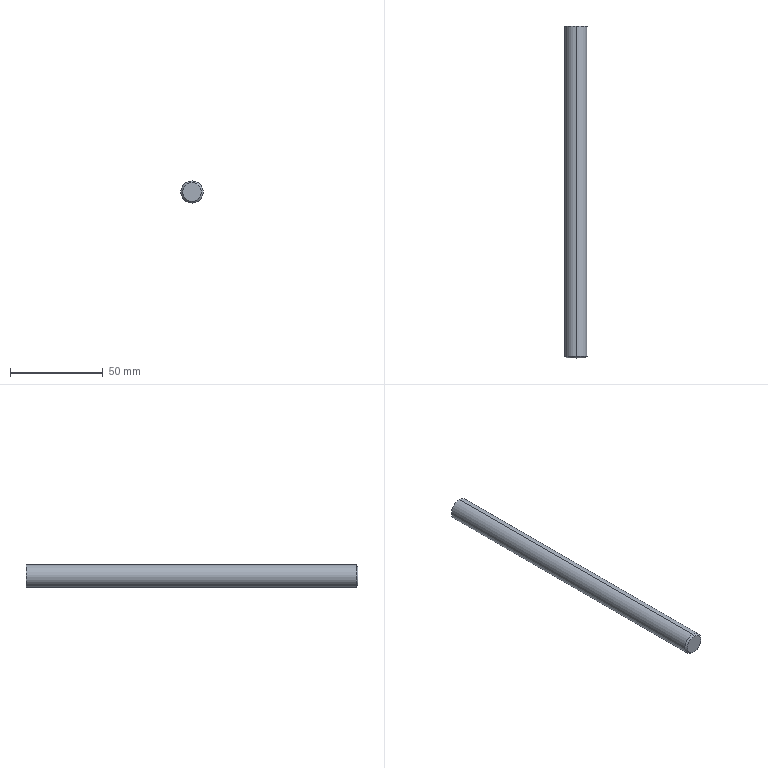Part | SolidWorks | features Chamfer 1, Extrusion 1, HoleWzd 1 | 1 solid | 10 faces | box 12 x 179 x 12 mm | volume 19967 mm3 | cone 4 | cylinder 4 | plane 2 | commonest cylinder face diameters 3.3 x2 12 x2
STEP:
#1=CARTESIAN_POINT('',(0.,0.,-5.));
#2=VERTEX_POINT('',#1);
#3=CARTESIAN_POINT('',(0.,0.,5.));
#4=VERTEX_POINT('',#3);
#5=CARTESIAN_POINT('',(0.,0.,0.));
#6=DIRECTION('',(0.,-1.,0.));
#7=DIRECTION('',(0.,0.,1.));
#8=AXIS2_PLACEMENT_3D('',#5,#6,#7);
#9=CIRCLE('',#8,5.);
#10=EDGE_CURVE('',#2,#4,#9,.T.);
#11=ORIENTED_EDGE('',*,*,#10,.F.);
#12=CARTESIAN_POINT('',(0.,1.,-6.));
#13=VERTEX_POINT('',#12);
#14=CARTESIAN_POINT('',(0.,1.,-6.));
#15=DIRECTION('',(0.,0.7071,-0.7071));
#16=VECTOR('',#15,1000.);
#17=LINE('',#14,#16);
#18=EDGE_CURVE('',#2,#13,#17,.T.);
#19=ORIENTED_EDGE('',*,*,#18,.T.);
#20=CARTESIAN_POINT('',(0.,1.,6.));
#21=VERTEX_POINT('',#20);
#22=CARTESIAN_POINT('',(0.,1.,0.));
#23=DIRECTION('',(0.,1.,0.));
#24=DIRECTION('',(0.,0.,1.));
#25=AXIS2_PLACEMENT_3D('',#22,#23,#24);
#26=CIRCLE('',#25,6.);
#27=EDGE_CURVE('',#21,#13,#26,.T.);
#28=ORIENTED_EDGE('',*,*,#27,.F.);
#29=CARTESIAN_POINT('',(0.,1.,6.));
#30=DIRECTION('',(0.,0.7071,0.7071));
#31=VECTOR('',#30,1000.);
#32=LINE('',#29,#31);
#33=EDGE_CURVE('',#4,#21,#32,.T.);
#34=ORIENTED_EDGE('',*,*,#33,.F.);
#35=EDGE_LOOP('',(#11,#19,#28,#34));
#36=FACE_OUTER_BOUND('',#35,.T.);
#37=CARTESIAN_POINT('',(0.,1.,0.));
#38=DIRECTION('',(0.,1.,0.));
#39=DIRECTION('',(0.,0.,1.));
#40=AXIS2_PLACEMENT_3D('',#37,#38,#39);
#41=CONICAL_SURFACE('',#40,6.,0.7854);
#42=ADVANCED_FACE('',(#36),#41,.T.);
#43=CARTESIAN_POINT('',(0.,149.,-1.65));
#44=VERTEX_POINT('',#43);
#45=CARTESIAN_POINT('',(0.,149.,1.65));
#46=VERTEX_POINT('',#45);
#47=CARTESIAN_POINT('',(0.,149.,0.));
#48=DIRECTION('',(0.,1.,0.));
#49=DIRECTION('',(0.,0.,1.));
#50=AXIS2_PLACEMENT_3D('',#47,#48,#49);
#51=CIRCLE('',#50,1.65);
#52=EDGE_CURVE('',#44,#46,#51,.T.);
#53=ORIENTED_EDGE('',*,*,#52,.F.);
#54=CARTESIAN_POINT('',(0.,179.,-1.65));
#55=VERTEX_POINT('',#54);
#56=CARTESIAN_POINT('',(0.,179.,-1.65));
#57=DIRECTION('',(0.,1.,0.));
#58=VECTOR('',#57,1000.);
#59=LINE('',#56,#58);
#60=EDGE_CURVE('',#44,#55,#59,.T.);
#61=ORIENTED_EDGE('',*,*,#60,.T.);
#62=CARTESIAN_POINT('',(0.,179.,1.65));
#63=VERTEX_POINT('',#62);
#64=CARTESIAN_POINT('',(0.,179.,0.));
#65=DIRECTION('',(0.,1.,0.));
#66=DIRECTION('',(0.,0.,1.));
#67=AXIS2_PLACEMENT_3D('',#64,#65,#66);
#68=CIRCLE('',#67,1.65);
#69=EDGE_CURVE('',#55,#63,#68,.T.);
#70=ORIENTED_EDGE('',*,*,#69,.T.);
#71=CARTESIAN_POINT('',(0.,179.,1.65));
#72=DIRECTION('',(0.,1.,0.));
#73=VECTOR('',#72,1000.);
#74=LINE('',#71,#73);
#75=EDGE_CURVE('',#46,#63,#74,.T.);
#76=ORIENTED_EDGE('',*,*,#75,.F.);
#77=EDGE_LOOP('',(#53,#61,#70,#76));
#78=FACE_OUTER_BOUND('',#77,.T.);
#79=CARTESIAN_POINT('',(0.,179.,0.));
#80=DIRECTION('',(0.,1.,0.));
#81=DIRECTION('',(0.,0.,1.));
#82=AXIS2_PLACEMENT_3D('',#79,#80,#81);
#83=CYLINDRICAL_SURFACE('',#82,1.65);
#84=ADVANCED_FACE('',(#78),#83,.F.);
#85=CARTESIAN_POINT('',(0.,148.009,0.));
#86=VERTEX_POINT('',#85);
#87=CARTESIAN_POINT('',(0.,149.,1.65));
#88=DIRECTION('',(0.,0.515,0.8572));
#89=VECTOR('',#88,1000.);
#90=LINE('',#87,#89);
#91=EDGE_CURVE('',#86,#46,#90,.T.);
#92=ORIENTED_EDGE('',*,*,#91,.F.);
#93=CARTESIAN_POINT('',(0.,149.,-1.65));
#94=DIRECTION('',(0.,0.515,-0.8572));
#95=VECTOR('',#94,1000.);
#96=LINE('',#93,#95);
#97=EDGE_CURVE('',#86,#44,#96,.T.);
#98=ORIENTED_EDGE('',*,*,#97,.T.);
#99=ORIENTED_EDGE('',*,*,#52,.T.);
#100=EDGE_LOOP('',(#92,#98,#99));
#101=FACE_OUTER_BOUND('',#100,.T.);
#102=CARTESIAN_POINT('',(0.,149.,0.));
#103=DIRECTION('',(0.,1.,0.));
#104=DIRECTION('',(0.,0.,1.));
#105=AXIS2_PLACEMENT_3D('',#102,#103,#104);
#106=CONICAL_SURFACE('',#105,1.65,1.03);
#107=ADVANCED_FACE('',(#101),#106,.F.);
#108=CARTESIAN_POINT('',(0.,179.,6.));
#109=VERTEX_POINT('',#108);
#110=CARTESIAN_POINT('',(0.,179.,-6.));
#111=VERTEX_POINT('',#110);
#112=CARTESIAN_POINT('',(0.,179.,0.));
#113=DIRECTION('',(0.,1.,0.));
#114=DIRECTION('',(0.,0.,1.));
#115=AXIS2_PLACEMENT_3D('',#112,#113,#114);
#116=CIRCLE('',#115,6.);
#117=EDGE_CURVE('',#109,#111,#116,.T.);
#118=ORIENTED_EDGE('',*,*,#117,.F.);
#119=CARTESIAN_POINT('',(0.,179.,6.));
#120=DIRECTION('',(0.,-1.,0.));
#121=VECTOR('',#120,1000.);
#122=LINE('',#119,#121);
#123=EDGE_CURVE('',#109,#21,#122,.T.);
#124=ORIENTED_EDGE('',*,*,#123,.T.);
#125=ORIENTED_EDGE('',*,*,#27,.T.);
#126=CARTESIAN_POINT('',(0.,179.,-6.));
#127=DIRECTION('',(0.,-1.,0.));
#128=VECTOR('',#127,1000.);
#129=LINE('',#126,#128);
#130=EDGE_CURVE('',#111,#13,#129,.T.);
#131=ORIENTED_EDGE('',*,*,#130,.F.);
#132=EDGE_LOOP('',(#118,#124,#125,#131));
#133=FACE_OUTER_BOUND('',#132,.T.);
#134=CARTESIAN_POINT('',(0.,179.,0.));
#135=DIRECTION('',(0.,-1.,0.));
#136=DIRECTION('',(0.,0.,-1.));
#137=AXIS2_PLACEMENT_3D('',#134,#135,#136);
#138=CYLINDRICAL_SURFACE('',#137,6.);
#139=ADVANCED_FACE('',(#133),#138,.T.);
#140=ORIENTED_EDGE('',*,*,#123,.F.);
#141=CARTESIAN_POINT('',(0.,179.,0.));
#142=DIRECTION('',(0.,1.,0.));
#143=DIRECTION('',(0.,0.,1.));
#144=AXIS2_PLACEMENT_3D('',#141,#142,#143);
#145=CIRCLE('',#144,6.);
#146=EDGE_CURVE('',#111,#109,#145,.T.);
#147=ORIENTED_EDGE('',*,*,#146,.F.);
#148=ORIENTED_EDGE('',*,*,#130,.T.);
#149=CARTESIAN_POINT('',(0.,1.,0.));
#150=DIRECTION('',(0.,1.,0.));
#151=DIRECTION('',(0.,0.,1.));
#152=AXIS2_PLACEMENT_3D('',#149,#150,#151);
#153=CIRCLE('',#152,6.);
#154=EDGE_CURVE('',#13,#21,#153,.T.);
#155=ORIENTED_EDGE('',*,*,#154,.T.);
#156=EDGE_LOOP('',(#140,#147,#148,#155));
#157=FACE_OUTER_BOUND('',#156,.T.);
#158=CARTESIAN_POINT('',(0.,179.,0.));
#159=DIRECTION('',(0.,-1.,0.));
#160=DIRECTION('',(0.,0.,-1.));
#161=AXIS2_PLACEMENT_3D('',#158,#159,#160);
#162=CYLINDRICAL_SURFACE('',#161,6.);
#163=ADVANCED_FACE('',(#157),#162,.T.);
#164=CARTESIAN_POINT('',(0.,179.,0.));
#165=DIRECTION('',(0.,1.,0.));
#166=DIRECTION('',(0.,0.,1.));
#167=AXIS2_PLACEMENT_3D('',#164,#165,#166);
#168=CIRCLE('',#167,1.65);
#169=EDGE_CURVE('',#63,#55,#168,.T.);
#170=ORIENTED_EDGE('',*,*,#169,.F.);
#171=ORIENTED_EDGE('',*,*,#69,.F.);
#172=EDGE_LOOP('',(#170,#171));
#173=FACE_BOUND('',#172,.T.);
#174=ORIENTED_EDGE('',*,*,#146,.T.);
#175=ORIENTED_EDGE('',*,*,#117,.T.);
#176=EDGE_LOOP('',(#174,#175));
#177=FACE_OUTER_BOUND('',#176,.T.);
#178=CARTESIAN_POINT('',(0.,179.,0.));
#179=DIRECTION('',(0.,1.,0.));
#180=DIRECTION('',(0.,0.,1.));
#181=AXIS2_PLACEMENT_3D('',#178,#179,#180);
#182=PLANE('',#181);
#183=ADVANCED_FACE('',(#173,#177),#182,.T.);
#184=CARTESIAN_POINT('',(0.,0.,0.));
#185=DIRECTION('',(0.,-1.,0.));
#186=DIRECTION('',(0.,0.,1.));
#187=AXIS2_PLACEMENT_3D('',#184,#185,#186);
#188=CIRCLE('',#187,5.);
#189=EDGE_CURVE('',#4,#2,#188,.T.);
#190=ORIENTED_EDGE('',*,*,#189,.T.);
#191=ORIENTED_EDGE('',*,*,#10,.T.);
#192=EDGE_LOOP('',(#190,#191));
#193=FACE_OUTER_BOUND('',#192,.T.);
#194=CARTESIAN_POINT('',(0.,0.,0.));
#195=DIRECTION('',(0.,1.,0.));
#196=DIRECTION('',(0.,0.,1.));
#197=AXIS2_PLACEMENT_3D('',#194,#195,#196);
#198=PLANE('',#197);
#199=ADVANCED_FACE('',(#193),#198,.F.);
#200=ORIENTED_EDGE('',*,*,#97,.F.);
#201=ORIENTED_EDGE('',*,*,#91,.T.);
#202=CARTESIAN_POINT('',(0.,149.,0.));
#203=DIRECTION('',(0.,1.,0.));
#204=DIRECTION('',(0.,0.,1.));
#205=AXIS2_PLACEMENT_3D('',#202,#203,#204);
#206=CIRCLE('',#205,1.65);
#207=EDGE_CURVE('',#46,#44,#206,.T.);
#208=ORIENTED_EDGE('',*,*,#207,.T.);
#209=EDGE_LOOP('',(#200,#201,#208));
#210=FACE_OUTER_BOUND('',#209,.T.);
#211=CARTESIAN_POINT('',(0.,149.,0.));
#212=DIRECTION('',(0.,1.,0.));
#213=DIRECTION('',(0.,0.,1.));
#214=AXIS2_PLACEMENT_3D('',#211,#212,#213);
#215=CONICAL_SURFACE('',#214,1.65,1.03);
#216=ADVANCED_FACE('',(#210),#215,.F.);
#217=ORIENTED_EDGE('',*,*,#60,.F.);
#218=ORIENTED_EDGE('',*,*,#207,.F.);
#219=ORIENTED_EDGE('',*,*,#75,.T.);
#220=ORIENTED_EDGE('',*,*,#169,.T.);
#221=EDGE_LOOP('',(#217,#218,#219,#220));
#222=FACE_OUTER_BOUND('',#221,.T.);
#223=CARTESIAN_POINT('',(0.,179.,0.));
#224=DIRECTION('',(0.,1.,0.));
#225=DIRECTION('',(0.,0.,1.));
#226=AXIS2_PLACEMENT_3D('',#223,#224,#225);
#227=CYLINDRICAL_SURFACE('',#226,1.65);
#228=ADVANCED_FACE('',(#222),#227,.F.);
#229=ORIENTED_EDGE('',*,*,#18,.F.);
#230=ORIENTED_EDGE('',*,*,#189,.F.);
#231=ORIENTED_EDGE('',*,*,#33,.T.);
#232=ORIENTED_EDGE('',*,*,#154,.F.);
#233=EDGE_LOOP('',(#229,#230,#231,#232));
#234=FACE_OUTER_BOUND('',#233,.T.);
#235=CARTESIAN_POINT('',(0.,1.,0.));
#236=DIRECTION('',(0.,1.,0.));
#237=DIRECTION('',(0.,0.,1.));
#238=AXIS2_PLACEMENT_3D('',#235,#236,#237);
#239=CONICAL_SURFACE('',#238,6.,0.7854);
#240=ADVANCED_FACE('',(#234),#239,.T.);
#241=CLOSED_SHELL('',(#42,#84,#107,#139,#163,#183,#199,#216,#228,#240));
#242=MANIFOLD_SOLID_BREP('',#241);
#243=CARTESIAN_POINT('',(0.,0.,0.));
#244=DIRECTION('',(0.,0.,1.));
#245=DIRECTION('',(1.,0.,0.));
#246=AXIS2_PLACEMENT_3D('',#243,#244,#245);
#247=(LENGTH_UNIT()NAMED_UNIT(*)SI_UNIT(.MILLI.,.METRE.));
#248=UNCERTAINTY_MEASURE_WITH_UNIT(LENGTH_MEASURE(0.00001),#247,'','');
#249=(NAMED_UNIT(*)PLANE_ANGLE_UNIT()SI_UNIT($,.RADIAN.));
#250=(NAMED_UNIT(*)SI_UNIT($,.STERADIAN.)SOLID_ANGLE_UNIT());
#251=(GEOMETRIC_REPRESENTATION_CONTEXT(3)GLOBAL_UNCERTAINTY_ASSIGNED_CONTEXT((#248))GLOBAL_UNIT_ASSIGNED_CONTEXT((#247,#249,#250))REPRESENTATION_CONTEXT('',''));
#252=ADVANCED_BREP_SHAPE_REPRESENTATION('',(#242,#246),#251);